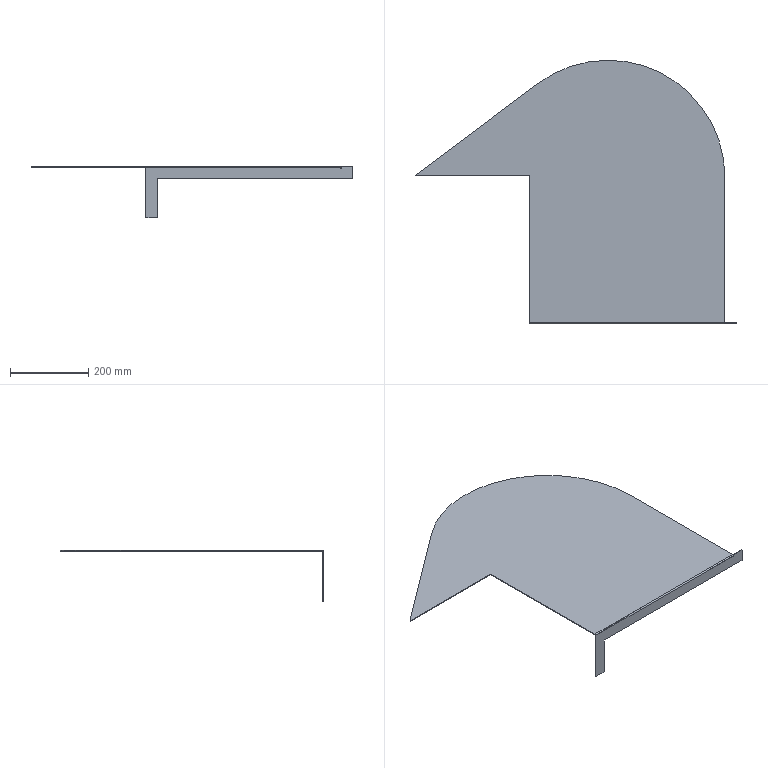Part | SolidWorks | features ICE 5, DeleteBody 3, Split 3, CombineBodies 1, Extrusion 1, FlatPattern 1, SheetMetal 1, Shell 1, SolidToSheetMetal 1 | 1 solid | 22 faces | box 823.333 x 675 x 132 mm | volume 728370 mm3 | plane 19 | cylinder 3 | commonest cylinder face diameters 2 x1 6 x1 600 x1
STEP:
#1=CARTESIAN_POINT('',(-500.,3.,-198.));
#2=VERTEX_POINT('',#1);
#3=CARTESIAN_POINT('',(-500.,3.,-200.));
#4=VERTEX_POINT('',#3);
#5=CARTESIAN_POINT('',(-500.,3.,-200.));
#6=DIRECTION('',(0.,0.,-1.));
#7=VECTOR('',#6,1000.);
#8=LINE('',#5,#7);
#9=EDGE_CURVE('',#2,#4,#8,.T.);
#10=ORIENTED_EDGE('',*,*,#9,.F.);
#11=CARTESIAN_POINT('',(-500.,380.,-198.));
#12=VERTEX_POINT('',#11);
#13=CARTESIAN_POINT('',(-500.,100.,-198.));
#14=DIRECTION('',(0.,-1.,0.));
#15=VECTOR('',#14,1000.);
#16=LINE('',#13,#15);
#17=EDGE_CURVE('',#12,#2,#16,.T.);
#18=ORIENTED_EDGE('',*,*,#17,.F.);
#19=CARTESIAN_POINT('',(-500.,380.,-200.));
#20=VERTEX_POINT('',#19);
#21=CARTESIAN_POINT('',(-500.,380.,-200.));
#22=DIRECTION('',(0.,0.,-1.));
#23=VECTOR('',#22,1000.);
#24=LINE('',#21,#23);
#25=EDGE_CURVE('',#12,#20,#24,.T.);
#26=ORIENTED_EDGE('',*,*,#25,.T.);
#27=CARTESIAN_POINT('',(-500.,380.,-200.));
#28=DIRECTION('',(0.,-1.,0.));
#29=VECTOR('',#28,1000.);
#30=LINE('',#27,#29);
#31=EDGE_CURVE('',#20,#4,#30,.T.);
#32=ORIENTED_EDGE('',*,*,#31,.T.);
#33=EDGE_LOOP('',(#10,#18,#26,#32));
#34=FACE_OUTER_BOUND('',#33,.T.);
#35=CARTESIAN_POINT('',(-500.,380.,-200.));
#36=DIRECTION('',(-1.,0.,0.));
#37=DIRECTION('',(0.,-1.,0.));
#38=AXIS2_PLACEMENT_3D('',#35,#36,#37);
#39=PLANE('',#38);
#40=ADVANCED_FACE('',(#34),#39,.T.);
#41=ORIENTED_EDGE('',*,*,#25,.F.);
#42=CARTESIAN_POINT('',(-793.333,380.,-198.));
#43=VERTEX_POINT('',#42);
#44=CARTESIAN_POINT('',(-1000.,380.,-198.));
#45=DIRECTION('',(-1.,0.,0.));
#46=VECTOR('',#45,1000.);
#47=LINE('',#44,#46);
#48=EDGE_CURVE('',#12,#43,#47,.T.);
#49=ORIENTED_EDGE('',*,*,#48,.T.);
#50=CARTESIAN_POINT('',(-793.333,380.,-200.));
#51=VERTEX_POINT('',#50);
#52=CARTESIAN_POINT('',(-793.333,380.,-200.));
#53=DIRECTION('',(0.,0.,-1.));
#54=VECTOR('',#53,1000.);
#55=LINE('',#52,#54);
#56=EDGE_CURVE('',#43,#51,#55,.T.);
#57=ORIENTED_EDGE('',*,*,#56,.T.);
#58=CARTESIAN_POINT('',(-1000.,380.,-200.));
#59=DIRECTION('',(-1.,0.,0.));
#60=VECTOR('',#59,1000.);
#61=LINE('',#58,#60);
#62=EDGE_CURVE('',#20,#51,#61,.T.);
#63=ORIENTED_EDGE('',*,*,#62,.F.);
#64=EDGE_LOOP('',(#41,#49,#57,#63));
#65=FACE_OUTER_BOUND('',#64,.T.);
#66=CARTESIAN_POINT('',(-1000.,380.,-200.));
#67=DIRECTION('',(0.,1.,0.));
#68=DIRECTION('',(-1.,0.,0.));
#69=AXIS2_PLACEMENT_3D('',#66,#67,#68);
#70=PLANE('',#69);
#71=ADVANCED_FACE('',(#65),#70,.F.);
#72=ORIENTED_EDGE('',*,*,#56,.F.);
#73=CARTESIAN_POINT('',(-480.,615.,-198.));
#74=VERTEX_POINT('',#73);
#75=CARTESIAN_POINT('',(-1060.,180.,-198.));
#76=DIRECTION('',(-0.8,-0.6,0.));
#77=VECTOR('',#76,1000.);
#78=LINE('',#75,#77);
#79=EDGE_CURVE('',#74,#43,#78,.T.);
#80=ORIENTED_EDGE('',*,*,#79,.F.);
#81=CARTESIAN_POINT('',(-480.,615.,-200.));
#82=VERTEX_POINT('',#81);
#83=CARTESIAN_POINT('',(-480.,615.,-200.));
#84=DIRECTION('',(0.,0.,-1.));
#85=VECTOR('',#84,1000.);
#86=LINE('',#83,#85);
#87=EDGE_CURVE('',#74,#82,#86,.T.);
#88=ORIENTED_EDGE('',*,*,#87,.T.);
#89=CARTESIAN_POINT('',(-1060.,180.,-200.));
#90=DIRECTION('',(-0.8,-0.6,0.));
#91=VECTOR('',#90,1000.);
#92=LINE('',#89,#91);
#93=EDGE_CURVE('',#82,#51,#92,.T.);
#94=ORIENTED_EDGE('',*,*,#93,.T.);
#95=EDGE_LOOP('',(#72,#80,#88,#94));
#96=FACE_OUTER_BOUND('',#95,.T.);
#97=CARTESIAN_POINT('',(-1060.,180.,-200.));
#98=DIRECTION('',(-0.6,0.8,0.));
#99=DIRECTION('',(-0.8,-0.6,0.));
#100=AXIS2_PLACEMENT_3D('',#97,#98,#99);
#101=PLANE('',#100);
#102=ADVANCED_FACE('',(#96),#101,.T.);
#103=ORIENTED_EDGE('',*,*,#87,.F.);
#104=CARTESIAN_POINT('',(0.,375.,-198.));
#105=VERTEX_POINT('',#104);
#106=CARTESIAN_POINT('',(-300.,375.,-198.));
#107=DIRECTION('',(0.,0.,1.));
#108=DIRECTION('',(1.,0.,0.));
#109=AXIS2_PLACEMENT_3D('',#106,#107,#108);
#110=CIRCLE('',#109,300.);
#111=EDGE_CURVE('',#105,#74,#110,.T.);
#112=ORIENTED_EDGE('',*,*,#111,.F.);
#113=CARTESIAN_POINT('',(0.,375.,-200.));
#114=VERTEX_POINT('',#113);
#115=CARTESIAN_POINT('',(0.,375.,-200.));
#116=DIRECTION('',(0.,0.,-1.));
#117=VECTOR('',#116,1000.);
#118=LINE('',#115,#117);
#119=EDGE_CURVE('',#105,#114,#118,.T.);
#120=ORIENTED_EDGE('',*,*,#119,.T.);
#121=CARTESIAN_POINT('',(-300.,375.,-200.));
#122=DIRECTION('',(0.,0.,1.));
#123=DIRECTION('',(1.,0.,0.));
#124=AXIS2_PLACEMENT_3D('',#121,#122,#123);
#125=CIRCLE('',#124,300.);
#126=EDGE_CURVE('',#114,#82,#125,.T.);
#127=ORIENTED_EDGE('',*,*,#126,.T.);
#128=EDGE_LOOP('',(#103,#112,#120,#127));
#129=FACE_OUTER_BOUND('',#128,.T.);
#130=CARTESIAN_POINT('',(-300.,375.,-200.));
#131=DIRECTION('',(0.,0.,1.));
#132=DIRECTION('',(1.,0.,0.));
#133=AXIS2_PLACEMENT_3D('',#130,#131,#132);
#134=CYLINDRICAL_SURFACE('',#133,300.);
#135=ADVANCED_FACE('',(#129),#134,.T.);
#136=ORIENTED_EDGE('',*,*,#119,.F.);
#137=CARTESIAN_POINT('',(0.,3.,-198.));
#138=VERTEX_POINT('',#137);
#139=CARTESIAN_POINT('',(0.,100.,-198.));
#140=DIRECTION('',(0.,1.,0.));
#141=VECTOR('',#140,1000.);
#142=LINE('',#139,#141);
#143=EDGE_CURVE('',#138,#105,#142,.T.);
#144=ORIENTED_EDGE('',*,*,#143,.F.);
#145=CARTESIAN_POINT('',(0.,3.,-200.));
#146=VERTEX_POINT('',#145);
#147=CARTESIAN_POINT('',(0.,3.,-200.));
#148=DIRECTION('',(0.,0.,-1.));
#149=VECTOR('',#148,1000.);
#150=LINE('',#147,#149);
#151=EDGE_CURVE('',#138,#146,#150,.T.);
#152=ORIENTED_EDGE('',*,*,#151,.T.);
#153=CARTESIAN_POINT('',(0.,0.,-200.));
#154=DIRECTION('',(0.,1.,0.));
#155=VECTOR('',#154,1000.);
#156=LINE('',#153,#155);
#157=EDGE_CURVE('',#146,#114,#156,.T.);
#158=ORIENTED_EDGE('',*,*,#157,.T.);
#159=EDGE_LOOP('',(#136,#144,#152,#158));
#160=FACE_OUTER_BOUND('',#159,.T.);
#161=CARTESIAN_POINT('',(0.,0.,-200.));
#162=DIRECTION('',(1.,0.,0.));
#163=DIRECTION('',(0.,1.,0.));
#164=AXIS2_PLACEMENT_3D('',#161,#162,#163);
#165=PLANE('',#164);
#166=ADVANCED_FACE('',(#160),#165,.T.);
#167=ORIENTED_EDGE('',*,*,#151,.F.);
#168=CARTESIAN_POINT('',(0.,0.,-201.));
#169=VERTEX_POINT('',#168);
#170=CARTESIAN_POINT('',(0.,3.,-201.));
#171=DIRECTION('',(1.,0.,0.));
#172=DIRECTION('',(0.,0.,1.));
#173=AXIS2_PLACEMENT_3D('',#170,#171,#172);
#174=CIRCLE('',#173,3.);
#175=EDGE_CURVE('',#138,#169,#174,.T.);
#176=ORIENTED_EDGE('',*,*,#175,.T.);
#177=CARTESIAN_POINT('',(0.,2.,-201.));
#178=VERTEX_POINT('',#177);
#179=CARTESIAN_POINT('',(0.,2.,-201.));
#180=DIRECTION('',(0.,1.,0.));
#181=VECTOR('',#180,1000.);
#182=LINE('',#179,#181);
#183=EDGE_CURVE('',#169,#178,#182,.T.);
#184=ORIENTED_EDGE('',*,*,#183,.T.);
#185=CARTESIAN_POINT('',(0.,3.,-201.));
#186=DIRECTION('',(1.,0.,0.));
#187=DIRECTION('',(0.,0.,1.));
#188=AXIS2_PLACEMENT_3D('',#185,#186,#187);
#189=CIRCLE('',#188,1.);
#190=EDGE_CURVE('',#146,#178,#189,.T.);
#191=ORIENTED_EDGE('',*,*,#190,.F.);
#192=EDGE_LOOP('',(#167,#176,#184,#191));
#193=FACE_OUTER_BOUND('',#192,.T.);
#194=CARTESIAN_POINT('',(0.,3.,-201.));
#195=DIRECTION('',(1.,0.,0.));
#196=DIRECTION('',(0.,0.,-1.));
#197=AXIS2_PLACEMENT_3D('',#194,#195,#196);
#198=PLANE('',#197);
#199=ADVANCED_FACE('',(#193),#198,.T.);
#200=ORIENTED_EDGE('',*,*,#183,.F.);
#201=CARTESIAN_POINT('',(0.,0.,-204.));
#202=VERTEX_POINT('',#201);
#203=CARTESIAN_POINT('',(0.,0.,0.));
#204=DIRECTION('',(0.,0.,1.));
#205=VECTOR('',#204,1000.);
#206=LINE('',#203,#205);
#207=EDGE_CURVE('',#202,#169,#206,.T.);
#208=ORIENTED_EDGE('',*,*,#207,.F.);
#209=CARTESIAN_POINT('',(0.,2.,-204.));
#210=VERTEX_POINT('',#209);
#211=CARTESIAN_POINT('',(0.,2.,-204.));
#212=DIRECTION('',(0.,1.,0.));
#213=VECTOR('',#212,1000.);
#214=LINE('',#211,#213);
#215=EDGE_CURVE('',#202,#210,#214,.T.);
#216=ORIENTED_EDGE('',*,*,#215,.T.);
#217=CARTESIAN_POINT('',(0.,2.,0.));
#218=DIRECTION('',(0.,0.,1.));
#219=VECTOR('',#218,1000.);
#220=LINE('',#217,#219);
#221=EDGE_CURVE('',#210,#178,#220,.T.);
#222=ORIENTED_EDGE('',*,*,#221,.T.);
#223=EDGE_LOOP('',(#200,#208,#216,#222));
#224=FACE_OUTER_BOUND('',#223,.T.);
#225=CARTESIAN_POINT('',(0.,2.,0.));
#226=DIRECTION('',(-1.,0.,0.));
#227=DIRECTION('',(0.,0.,1.));
#228=AXIS2_PLACEMENT_3D('',#225,#226,#227);
#229=PLANE('',#228);
#230=ADVANCED_FACE('',(#224),#229,.F.);
#231=ORIENTED_EDGE('',*,*,#215,.F.);
#232=CARTESIAN_POINT('',(1.,0.,-204.));
#233=VERTEX_POINT('',#232);
#234=CARTESIAN_POINT('',(0.,0.,-204.));
#235=DIRECTION('',(-1.,0.,0.));
#236=VECTOR('',#235,1000.);
#237=LINE('',#234,#236);
#238=EDGE_CURVE('',#233,#202,#237,.T.);
#239=ORIENTED_EDGE('',*,*,#238,.F.);
#240=CARTESIAN_POINT('',(1.,2.,-204.));
#241=VERTEX_POINT('',#240);
#242=CARTESIAN_POINT('',(1.,2.,-204.));
#243=DIRECTION('',(0.,1.,0.));
#244=VECTOR('',#243,1000.);
#245=LINE('',#242,#244);
#246=EDGE_CURVE('',#233,#241,#245,.T.);
#247=ORIENTED_EDGE('',*,*,#246,.T.);
#248=CARTESIAN_POINT('',(0.,2.,-204.));
#249=DIRECTION('',(-1.,0.,0.));
#250=VECTOR('',#249,1000.);
#251=LINE('',#248,#250);
#252=EDGE_CURVE('',#241,#210,#251,.T.);
#253=ORIENTED_EDGE('',*,*,#252,.T.);
#254=EDGE_LOOP('',(#231,#239,#247,#253));
#255=FACE_OUTER_BOUND('',#254,.T.);
#256=CARTESIAN_POINT('',(0.,2.,-204.));
#257=DIRECTION('',(0.,0.,-1.));
#258=DIRECTION('',(-1.,0.,0.));
#259=AXIS2_PLACEMENT_3D('',#256,#257,#258);
#260=PLANE('',#259);
#261=ADVANCED_FACE('',(#255),#260,.F.);
#262=ORIENTED_EDGE('',*,*,#246,.F.);
#263=CARTESIAN_POINT('',(1.,0.,-198.));
#264=VERTEX_POINT('',#263);
#265=CARTESIAN_POINT('',(1.,0.,0.));
#266=DIRECTION('',(0.,0.,-1.));
#267=VECTOR('',#266,1000.);
#268=LINE('',#265,#267);
#269=EDGE_CURVE('',#264,#233,#268,.T.);
#270=ORIENTED_EDGE('',*,*,#269,.F.);
#271=CARTESIAN_POINT('',(1.,2.,-198.));
#272=VERTEX_POINT('',#271);
#273=CARTESIAN_POINT('',(1.,2.,-198.));
#274=DIRECTION('',(0.,1.,0.));
#275=VECTOR('',#274,1000.);
#276=LINE('',#273,#275);
#277=EDGE_CURVE('',#264,#272,#276,.T.);
#278=ORIENTED_EDGE('',*,*,#277,.T.);
#279=CARTESIAN_POINT('',(1.,2.,0.));
#280=DIRECTION('',(0.,0.,-1.));
#281=VECTOR('',#280,1000.);
#282=LINE('',#279,#281);
#283=EDGE_CURVE('',#272,#241,#282,.T.);
#284=ORIENTED_EDGE('',*,*,#283,.T.);
#285=EDGE_LOOP('',(#262,#270,#278,#284));
#286=FACE_OUTER_BOUND('',#285,.T.);
#287=CARTESIAN_POINT('',(1.,2.,0.));
#288=DIRECTION('',(1.,0.,0.));
#289=DIRECTION('',(0.,0.,-1.));
#290=AXIS2_PLACEMENT_3D('',#287,#288,#289);
#291=PLANE('',#290);
#292=ADVANCED_FACE('',(#286),#291,.F.);
#293=ORIENTED_EDGE('',*,*,#277,.F.);
#294=CARTESIAN_POINT('',(30.,0.,-198.));
#295=VERTEX_POINT('',#294);
#296=CARTESIAN_POINT('',(0.,0.,-198.));
#297=DIRECTION('',(1.,0.,0.));
#298=VECTOR('',#297,1000.);
#299=LINE('',#296,#298);
#300=EDGE_CURVE('',#264,#295,#299,.T.);
#301=ORIENTED_EDGE('',*,*,#300,.T.);
#302=CARTESIAN_POINT('',(30.,2.,-198.));
#303=VERTEX_POINT('',#302);
#304=CARTESIAN_POINT('',(30.,2.,-198.));
#305=DIRECTION('',(0.,1.,0.));
#306=VECTOR('',#305,1000.);
#307=LINE('',#304,#306);
#308=EDGE_CURVE('',#295,#303,#307,.T.);
#309=ORIENTED_EDGE('',*,*,#308,.T.);
#310=CARTESIAN_POINT('',(0.,2.,-198.));
#311=DIRECTION('',(1.,0.,0.));
#312=VECTOR('',#311,1000.);
#313=LINE('',#310,#312);
#314=EDGE_CURVE('',#272,#303,#313,.T.);
#315=ORIENTED_EDGE('',*,*,#314,.F.);
#316=EDGE_LOOP('',(#293,#301,#309,#315));
#317=FACE_OUTER_BOUND('',#316,.T.);
#318=CARTESIAN_POINT('',(0.,2.,-198.));
#319=DIRECTION('',(0.,0.,1.));
#320=DIRECTION('',(1.,0.,0.));
#321=AXIS2_PLACEMENT_3D('',#318,#319,#320);
#322=PLANE('',#321);
#323=ADVANCED_FACE('',(#317),#322,.T.);
#324=ORIENTED_EDGE('',*,*,#308,.F.);
#325=CARTESIAN_POINT('',(30.,0.,-230.));
#326=VERTEX_POINT('',#325);
#327=CARTESIAN_POINT('',(30.,0.,0.));
#328=DIRECTION('',(0.,0.,1.));
#329=VECTOR('',#328,1000.);
#330=LINE('',#327,#329);
#331=EDGE_CURVE('',#326,#295,#330,.T.);
#332=ORIENTED_EDGE('',*,*,#331,.F.);
#333=CARTESIAN_POINT('',(30.,2.,-230.));
#334=VERTEX_POINT('',#333);
#335=CARTESIAN_POINT('',(30.,2.,-230.));
#336=DIRECTION('',(0.,1.,0.));
#337=VECTOR('',#336,1000.);
#338=LINE('',#335,#337);
#339=EDGE_CURVE('',#326,#334,#338,.T.);
#340=ORIENTED_EDGE('',*,*,#339,.T.);
#341=CARTESIAN_POINT('',(30.,2.,-230.));
#342=DIRECTION('',(0.,0.,1.));
#343=VECTOR('',#342,1000.);
#344=LINE('',#341,#343);
#345=EDGE_CURVE('',#334,#303,#344,.T.);
#346=ORIENTED_EDGE('',*,*,#345,.T.);
#347=EDGE_LOOP('',(#324,#332,#340,#346));
#348=FACE_OUTER_BOUND('',#347,.T.);
#349=CARTESIAN_POINT('',(30.,2.,-230.));
#350=DIRECTION('',(-1.,0.,0.));
#351=DIRECTION('',(0.,0.,1.));
#352=AXIS2_PLACEMENT_3D('',#349,#350,#351);
#353=PLANE('',#352);
#354=ADVANCED_FACE('',(#348),#353,.F.);
#355=ORIENTED_EDGE('',*,*,#339,.F.);
#356=CARTESIAN_POINT('',(-470.,0.,-230.));
#357=VERTEX_POINT('',#356);
#358=CARTESIAN_POINT('',(0.,0.,-230.));
#359=DIRECTION('',(1.,0.,0.));
#360=VECTOR('',#359,1000.);
#361=LINE('',#358,#360);
#362=EDGE_CURVE('',#357,#326,#361,.T.);
#363=ORIENTED_EDGE('',*,*,#362,.F.);
#364=CARTESIAN_POINT('',(-470.,2.,-230.));
#365=VERTEX_POINT('',#364);
#366=CARTESIAN_POINT('',(-470.,2.,-230.));
#367=DIRECTION('',(0.,1.,0.));
#368=VECTOR('',#367,1000.);
#369=LINE('',#366,#368);
#370=EDGE_CURVE('',#357,#365,#369,.T.);
#371=ORIENTED_EDGE('',*,*,#370,.T.);
#372=CARTESIAN_POINT('',(-470.,2.,-230.));
#373=DIRECTION('',(1.,0.,0.));
#374=VECTOR('',#373,1000.);
#375=LINE('',#372,#374);
#376=EDGE_CURVE('',#365,#334,#375,.T.);
#377=ORIENTED_EDGE('',*,*,#376,.T.);
#378=EDGE_LOOP('',(#355,#363,#371,#377));
#379=FACE_OUTER_BOUND('',#378,.T.);
#380=CARTESIAN_POINT('',(-470.,2.,-230.));
#381=DIRECTION('',(0.,0.,1.));
#382=DIRECTION('',(1.,0.,0.));
#383=AXIS2_PLACEMENT_3D('',#380,#381,#382);
#384=PLANE('',#383);
#385=ADVANCED_FACE('',(#379),#384,.F.);
#386=ORIENTED_EDGE('',*,*,#370,.F.);
#387=CARTESIAN_POINT('',(-470.,0.,-330.));
#388=VERTEX_POINT('',#387);
#389=CARTESIAN_POINT('',(-470.,0.,0.));
#390=DIRECTION('',(0.,0.,1.));
#391=VECTOR('',#390,1000.);
#392=LINE('',#389,#391);
#393=EDGE_CURVE('',#388,#357,#392,.T.);
#394=ORIENTED_EDGE('',*,*,#393,.F.);
#395=CARTESIAN_POINT('',(-470.,2.,-330.));
#396=VERTEX_POINT('',#395);
#397=CARTESIAN_POINT('',(-470.,2.,-330.));
#398=DIRECTION('',(0.,1.,0.));
#399=VECTOR('',#398,1000.);
#400=LINE('',#397,#399);
#401=EDGE_CURVE('',#388,#396,#400,.T.);
#402=ORIENTED_EDGE('',*,*,#401,.T.);
#403=CARTESIAN_POINT('',(-470.,2.,-330.));
#404=DIRECTION('',(0.,0.,1.));
#405=VECTOR('',#404,1000.);
#406=LINE('',#403,#405);
#407=EDGE_CURVE('',#396,#365,#406,.T.);
#408=ORIENTED_EDGE('',*,*,#407,.T.);
#409=EDGE_LOOP('',(#386,#394,#402,#408));
#410=FACE_OUTER_BOUND('',#409,.T.);
#411=CARTESIAN_POINT('',(-470.,2.,-330.));
#412=DIRECTION('',(-1.,0.,0.));
#413=DIRECTION('',(0.,0.,1.));
#414=AXIS2_PLACEMENT_3D('',#411,#412,#413);
#415=PLANE('',#414);
#416=ADVANCED_FACE('',(#410),#415,.F.);
#417=ORIENTED_EDGE('',*,*,#401,.F.);
#418=CARTESIAN_POINT('',(-500.,0.,-330.));
#419=VERTEX_POINT('',#418);
#420=CARTESIAN_POINT('',(0.,0.,-330.));
#421=DIRECTION('',(1.,0.,0.));
#422=VECTOR('',#421,1000.);
#423=LINE('',#420,#422);
#424=EDGE_CURVE('',#419,#388,#423,.T.);
#425=ORIENTED_EDGE('',*,*,#424,.F.);
#426=CARTESIAN_POINT('',(-500.,2.,-330.));
#427=VERTEX_POINT('',#426);
#428=CARTESIAN_POINT('',(-500.,2.,-330.));
#429=DIRECTION('',(0.,1.,0.));
#430=VECTOR('',#429,1000.);
#431=LINE('',#428,#430);
#432=EDGE_CURVE('',#419,#427,#431,.T.);
#433=ORIENTED_EDGE('',*,*,#432,.T.);
#434=CARTESIAN_POINT('',(-1130.,2.,-330.));
#435=DIRECTION('',(1.,0.,0.));
#436=VECTOR('',#435,1000.);
#437=LINE('',#434,#436);
#438=EDGE_CURVE('',#427,#396,#437,.T.);
#439=ORIENTED_EDGE('',*,*,#438,.T.);
#440=EDGE_LOOP('',(#417,#425,#433,#439));
#441=FACE_OUTER_BOUND('',#440,.T.);
#442=CARTESIAN_POINT('',(-1130.,2.,-330.));
#443=DIRECTION('',(0.,0.,1.));
#444=DIRECTION('',(1.,0.,0.));
#445=AXIS2_PLACEMENT_3D('',#442,#443,#444);
#446=PLANE('',#445);
#447=ADVANCED_FACE('',(#441),#446,.F.);
#448=ORIENTED_EDGE('',*,*,#432,.F.);
#449=CARTESIAN_POINT('',(-500.,0.,-201.));
#450=VERTEX_POINT('',#449);
#451=CARTESIAN_POINT('',(-500.,0.,0.));
#452=DIRECTION('',(0.,0.,-1.));
#453=VECTOR('',#452,1000.);
#454=LINE('',#451,#453);
#455=EDGE_CURVE('',#450,#419,#454,.T.);
#456=ORIENTED_EDGE('',*,*,#455,.F.);
#457=CARTESIAN_POINT('',(-500.,2.,-201.));
#458=VERTEX_POINT('',#457);
#459=CARTESIAN_POINT('',(-500.,2.,-201.));
#460=DIRECTION('',(0.,1.,0.));
#461=VECTOR('',#460,1000.);
#462=LINE('',#459,#461);
#463=EDGE_CURVE('',#450,#458,#462,.T.);
#464=ORIENTED_EDGE('',*,*,#463,.T.);
#465=CARTESIAN_POINT('',(-500.,2.,0.));
#466=DIRECTION('',(0.,0.,-1.));
#467=VECTOR('',#466,1000.);
#468=LINE('',#465,#467);
#469=EDGE_CURVE('',#458,#427,#468,.T.);
#470=ORIENTED_EDGE('',*,*,#469,.T.);
#471=EDGE_LOOP('',(#448,#456,#464,#470));
#472=FACE_OUTER_BOUND('',#471,.T.);
#473=CARTESIAN_POINT('',(-500.,2.,0.));
#474=DIRECTION('',(1.,0.,0.));
#475=DIRECTION('',(0.,0.,-1.));
#476=AXIS2_PLACEMENT_3D('',#473,#474,#475);
#477=PLANE('',#476);
#478=ADVANCED_FACE('',(#472),#477,.F.);
#479=CARTESIAN_POINT('',(-500.,3.,-201.));
#480=DIRECTION('',(-1.,0.,0.));
#481=DIRECTION('',(0.,0.,1.));
#482=AXIS2_PLACEMENT_3D('',#479,#480,#481);
#483=CIRCLE('',#482,3.);
#484=EDGE_CURVE('',#450,#2,#483,.T.);
#485=ORIENTED_EDGE('',*,*,#484,.T.);
#486=ORIENTED_EDGE('',*,*,#9,.T.);
#487=CARTESIAN_POINT('',(-500.,3.,-201.));
#488=DIRECTION('',(-1.,0.,0.));
#489=DIRECTION('',(0.,0.,-1.));
#490=AXIS2_PLACEMENT_3D('',#487,#488,#489);
#491=CIRCLE('',#490,1.);
#492=EDGE_CURVE('',#458,#4,#491,.T.);
#493=ORIENTED_EDGE('',*,*,#492,.F.);
#494=ORIENTED_EDGE('',*,*,#463,.F.);
#495=EDGE_LOOP('',(#485,#486,#493,#494));
#496=FACE_OUTER_BOUND('',#495,.T.);
#497=CARTESIAN_POINT('',(-500.,3.,-201.));
#498=DIRECTION('',(-1.,0.,0.));
#499=DIRECTION('',(0.,0.,1.));
#500=AXIS2_PLACEMENT_3D('',#497,#498,#499);
#501=PLANE('',#500);
#502=ADVANCED_FACE('',(#496),#501,.T.);
#503=ORIENTED_EDGE('',*,*,#469,.F.);
#504=CARTESIAN_POINT('',(0.,2.,-201.));
#505=DIRECTION('',(1.,0.,0.));
#506=VECTOR('',#505,1000.);
#507=LINE('',#504,#506);
#508=EDGE_CURVE('',#458,#178,#507,.T.);
#509=ORIENTED_EDGE('',*,*,#508,.T.);
#510=ORIENTED_EDGE('',*,*,#221,.F.);
#511=ORIENTED_EDGE('',*,*,#252,.F.);
#512=ORIENTED_EDGE('',*,*,#283,.F.);
#513=ORIENTED_EDGE('',*,*,#314,.T.);
#514=ORIENTED_EDGE('',*,*,#345,.F.);
#515=ORIENTED_EDGE('',*,*,#376,.F.);
#516=ORIENTED_EDGE('',*,*,#407,.F.);
#517=ORIENTED_EDGE('',*,*,#438,.F.);
#518=EDGE_LOOP('',(#503,#509,#510,#511,#512,#513,#514,#515,#516,#517));
#519=FACE_OUTER_BOUND('',#518,.T.);
#520=CARTESIAN_POINT('',(0.,2.,0.));
#521=DIRECTION('',(0.,1.,0.));
#522=DIRECTION('',(0.,0.,1.));
#523=AXIS2_PLACEMENT_3D('',#520,#521,#522);
#524=PLANE('',#523);
#525=ADVANCED_FACE('',(#519),#524,.T.);
#526=ORIENTED_EDGE('',*,*,#157,.F.);
#527=CARTESIAN_POINT('',(-1000.,3.,-200.));
#528=DIRECTION('',(-1.,0.,0.));
#529=VECTOR('',#528,1000.);
#530=LINE('',#527,#529);
#531=EDGE_CURVE('',#146,#4,#530,.T.);
#532=ORIENTED_EDGE('',*,*,#531,.T.);
#533=ORIENTED_EDGE('',*,*,#31,.F.);
#534=ORIENTED_EDGE('',*,*,#62,.T.);
#535=ORIENTED_EDGE('',*,*,#93,.F.);
#536=ORIENTED_EDGE('',*,*,#126,.F.);
#537=EDGE_LOOP('',(#526,#532,#533,#534,#535,#536));
#538=FACE_OUTER_BOUND('',#537,.T.);
#539=CARTESIAN_POINT('',(-1000.,100.,-200.));
#540=DIRECTION('',(0.,0.,1.));
#541=DIRECTION('',(1.,0.,0.));
#542=AXIS2_PLACEMENT_3D('',#539,#540,#541);
#543=PLANE('',#542);
#544=ADVANCED_FACE('',(#538),#543,.F.);
#545=ORIENTED_EDGE('',*,*,#190,.T.);
#546=ORIENTED_EDGE('',*,*,#508,.F.);
#547=ORIENTED_EDGE('',*,*,#492,.T.);
#548=ORIENTED_EDGE('',*,*,#531,.F.);
#549=EDGE_LOOP('',(#545,#546,#547,#548));
#550=FACE_OUTER_BOUND('',#549,.T.);
#551=CARTESIAN_POINT('',(-1000.,3.,-201.));
#552=DIRECTION('',(-1.,0.,0.));
#553=DIRECTION('',(0.,0.,1.));
#554=AXIS2_PLACEMENT_3D('',#551,#552,#553);
#555=CYLINDRICAL_SURFACE('',#554,1.);
#556=ADVANCED_FACE('',(#550),#555,.F.);
#557=ORIENTED_EDGE('',*,*,#455,.T.);
#558=ORIENTED_EDGE('',*,*,#424,.T.);
#559=ORIENTED_EDGE('',*,*,#393,.T.);
#560=ORIENTED_EDGE('',*,*,#362,.T.);
#561=ORIENTED_EDGE('',*,*,#331,.T.);
#562=ORIENTED_EDGE('',*,*,#300,.F.);
#563=ORIENTED_EDGE('',*,*,#269,.T.);
#564=ORIENTED_EDGE('',*,*,#238,.T.);
#565=ORIENTED_EDGE('',*,*,#207,.T.);
#566=CARTESIAN_POINT('',(0.,0.,-201.));
#567=DIRECTION('',(1.,0.,0.));
#568=VECTOR('',#567,1000.);
#569=LINE('',#566,#568);
#570=EDGE_CURVE('',#450,#169,#569,.T.);
#571=ORIENTED_EDGE('',*,*,#570,.F.);
#572=EDGE_LOOP('',(#557,#558,#559,#560,#561,#562,#563,#564,#565,#571));
#573=FACE_OUTER_BOUND('',#572,.T.);
#574=CARTESIAN_POINT('',(0.,0.,0.));
#575=DIRECTION('',(0.,1.,0.));
#576=DIRECTION('',(0.,0.,1.));
#577=AXIS2_PLACEMENT_3D('',#574,#575,#576);
#578=PLANE('',#577);
#579=ADVANCED_FACE('',(#573),#578,.F.);
#580=ORIENTED_EDGE('',*,*,#143,.T.);
#581=ORIENTED_EDGE('',*,*,#111,.T.);
#582=ORIENTED_EDGE('',*,*,#79,.T.);
#583=ORIENTED_EDGE('',*,*,#48,.F.);
#584=ORIENTED_EDGE('',*,*,#17,.T.);
#585=CARTESIAN_POINT('',(-1000.,3.,-198.));
#586=DIRECTION('',(-1.,0.,0.));
#587=VECTOR('',#586,1000.);
#588=LINE('',#585,#587);
#589=EDGE_CURVE('',#138,#2,#588,.T.);
#590=ORIENTED_EDGE('',*,*,#589,.F.);
#591=EDGE_LOOP('',(#580,#581,#582,#583,#584,#590));
#592=FACE_OUTER_BOUND('',#591,.T.);
#593=CARTESIAN_POINT('',(-1000.,100.,-198.));
#594=DIRECTION('',(0.,0.,1.));
#595=DIRECTION('',(1.,0.,0.));
#596=AXIS2_PLACEMENT_3D('',#593,#594,#595);
#597=PLANE('',#596);
#598=ADVANCED_FACE('',(#592),#597,.T.);
#599=ORIENTED_EDGE('',*,*,#175,.F.);
#600=ORIENTED_EDGE('',*,*,#589,.T.);
#601=ORIENTED_EDGE('',*,*,#484,.F.);
#602=ORIENTED_EDGE('',*,*,#570,.T.);
#603=EDGE_LOOP('',(#599,#600,#601,#602));
#604=FACE_OUTER_BOUND('',#603,.T.);
#605=CARTESIAN_POINT('',(-1000.,3.,-201.));
#606=DIRECTION('',(-1.,0.,0.));
#607=DIRECTION('',(0.,0.,1.));
#608=AXIS2_PLACEMENT_3D('',#605,#606,#607);
#609=CYLINDRICAL_SURFACE('',#608,3.);
#610=ADVANCED_FACE('',(#604),#609,.T.);
#611=CLOSED_SHELL('',(#40,#71,#102,#135,#166,#199,#230,#261,#292,#323,#354,#385,#416,#447,#478,#502,#525,#544,#556,#579,#598,#610));
#612=MANIFOLD_SOLID_BREP('',#611);
#613=CARTESIAN_POINT('',(0.,0.,0.));
#614=DIRECTION('',(0.,0.,1.));
#615=DIRECTION('',(1.,0.,0.));
#616=AXIS2_PLACEMENT_3D('',#613,#614,#615);
#617=(LENGTH_UNIT()NAMED_UNIT(*)SI_UNIT(.MILLI.,.METRE.));
#618=UNCERTAINTY_MEASURE_WITH_UNIT(LENGTH_MEASURE(0.00001),#617,'','');
#619=(NAMED_UNIT(*)PLANE_ANGLE_UNIT()SI_UNIT($,.RADIAN.));
#620=(NAMED_UNIT(*)SI_UNIT($,.STERADIAN.)SOLID_ANGLE_UNIT());
#621=(GEOMETRIC_REPRESENTATION_CONTEXT(3)GLOBAL_UNCERTAINTY_ASSIGNED_CONTEXT((#618))GLOBAL_UNIT_ASSIGNED_CONTEXT((#617,#619,#620))REPRESENTATION_CONTEXT('',''));
#622=ADVANCED_BREP_SHAPE_REPRESENTATION('',(#612,#616),#621);